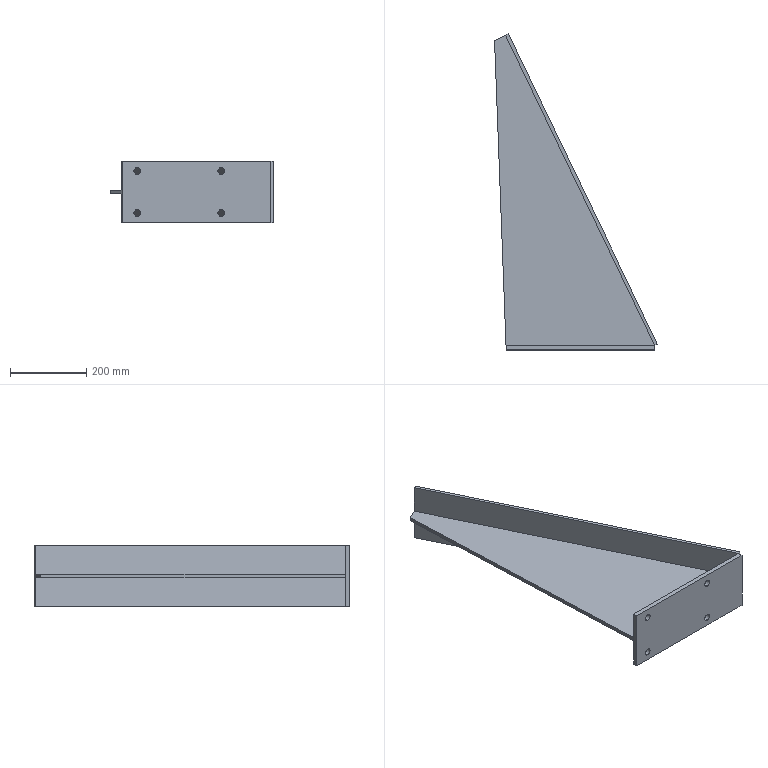Part | STEP file | Screen frame rear support_Default<As machined> | 3 solids | 26 faces | box 426.209 x 826.5 x 160 mm | volume 3581140 mm3 | plane 18 | cylinder 8 | commonest cylinder face diameters 18 x8